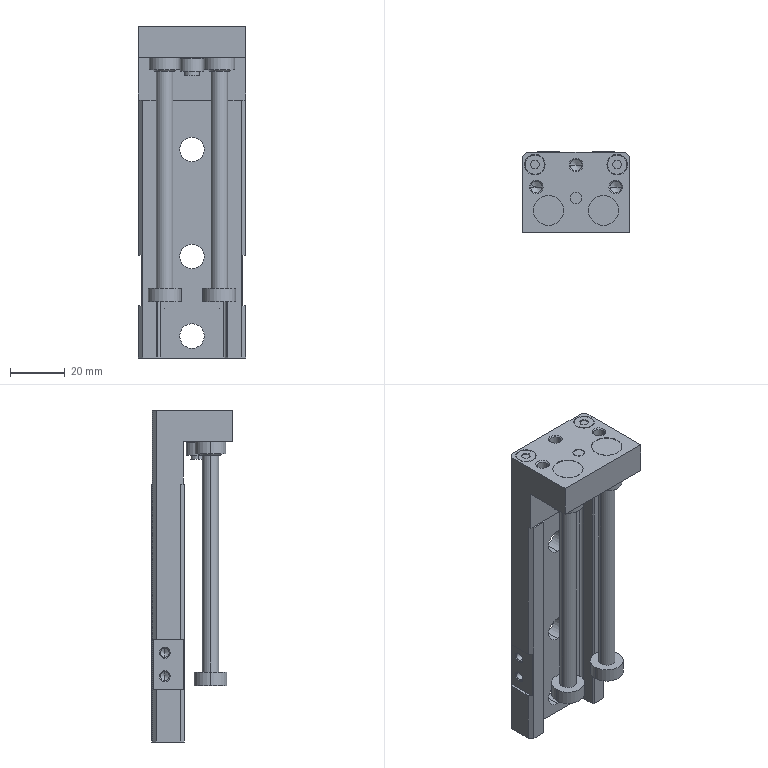Part | SolidWorks | features RefAxis 15, HoleWzd 11, ICE 9, 3DProfileFeature 5, LPattern 4, Revolution 3, RevCut 2, Extrusion 1 | 1 solid | 203 faces | box 39 x 29.5 x 121 mm | volume 53131 mm3 | plane 76 | cylinder 71 | cone 52 | torus 4 | commonest cylinder face diameters 3.242 x20 4.134 x6 9 x6 4 x5 6 x4 7 x4